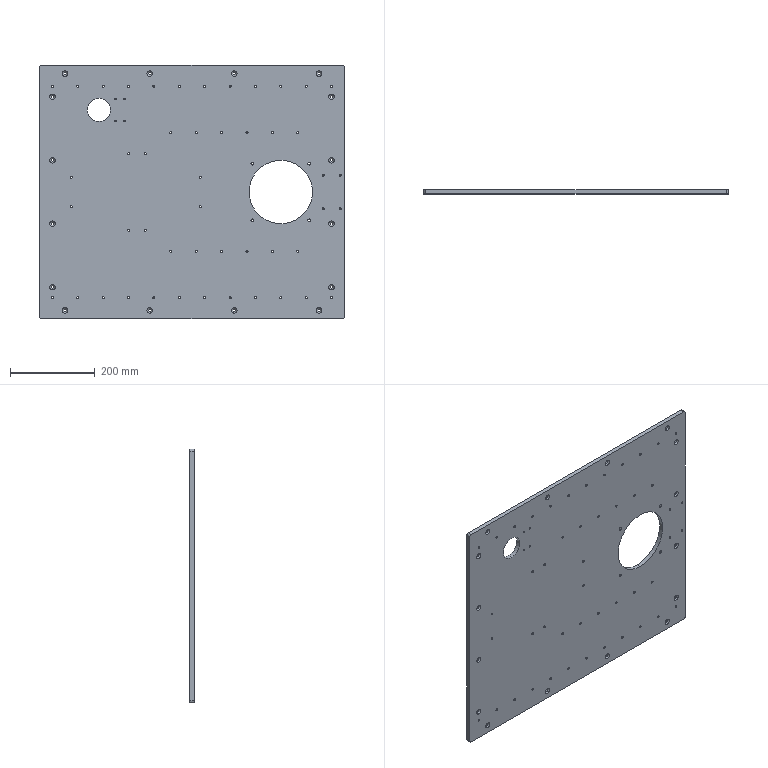Part | STEP file | Bracket二台Face Plate | 1 solid | 190 faces | box 720 x 10 x 600 mm | volume 4099998 mm3 | cylinder 152 | cone 32 | plane 6 | commonest cylinder face diameters 5 x96 6.6 x32 4.2 x8 6.8 x8 10 x4 55 x2